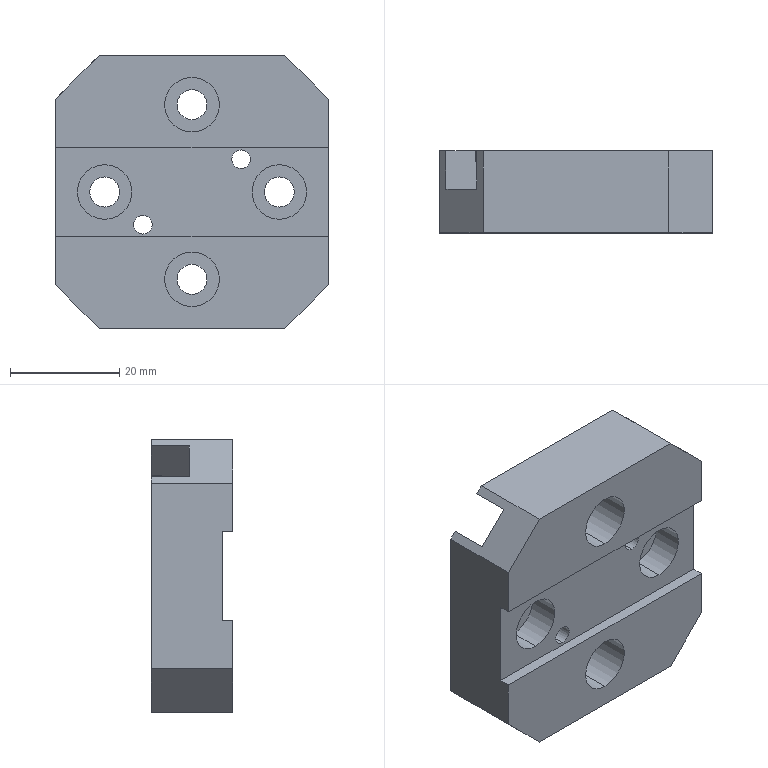Part | STEP file | PN_0004 | 1 solid | 52 faces | box 50 x 15 x 50 mm | volume 26390 mm3 | cylinder 28 | plane 24 | commonest cylinder face diameters 5.5 x8 10 x8 3.4 x4 6 x4 45 x3 8 x1